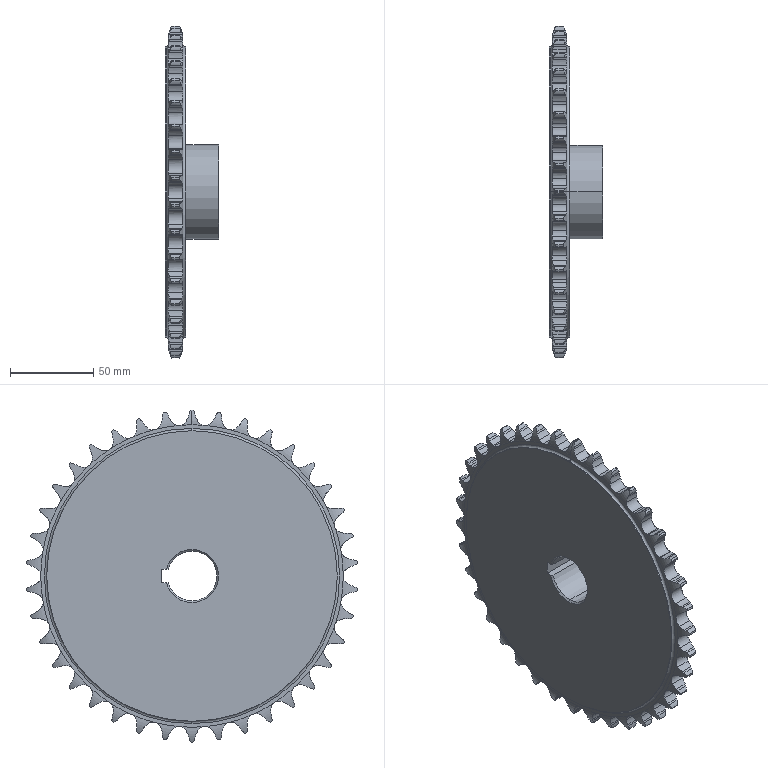Part | SolidWorks | features Chamfer 2, Cut 2, Revolution 2, CirPattern 1 | 1 solid | 428 faces | box 32 x 199.417 x 200 mm | volume 354136 mm3 | cylinder 256 | plane 84 | torus 82 | cone 6 | commonest cylinder face diameters 14.495 x80 26.567 x78 10.311 x50 200 x39 175 x4 30 x3